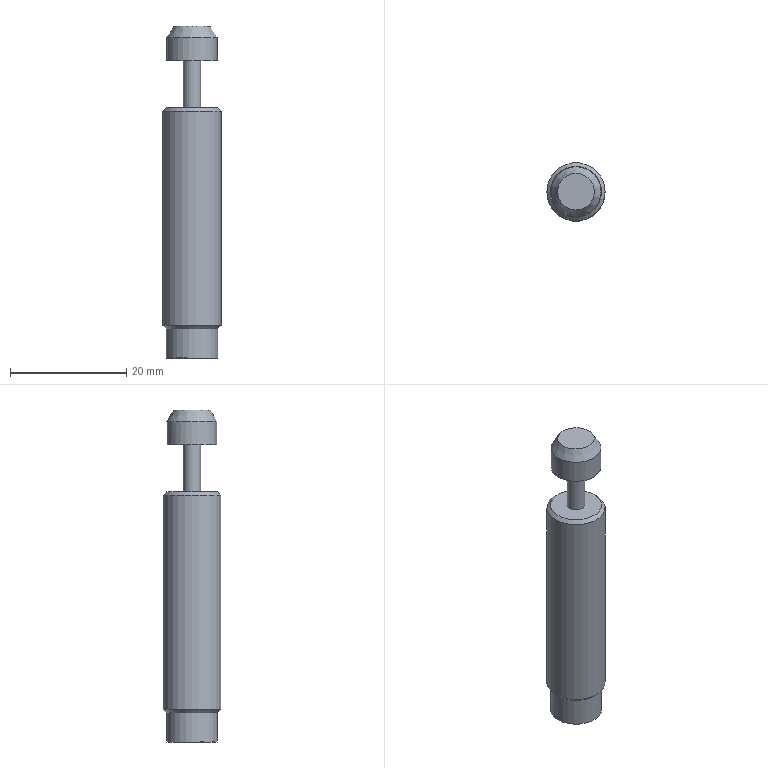Part | NX | 1 solid | 11 faces | box 10 x 10 x 57 mm | volume 3652 mm3 | cylinder 4 | plane 4 | cone 3 | commonest cylinder face diameters 3 x1 8.6 x1 8.773 x1 10 x1
STEP:
#1=CARTESIAN_POINT('',(-5.,0.,-0.6135));
#2=VERTEX_POINT('',#1);
#3=CARTESIAN_POINT('',(0.,0.,-0.6135));
#4=DIRECTION('',(0.,0.,1.));
#5=DIRECTION('',(1.,0.,0.));
#6=AXIS2_PLACEMENT_3D('',#3,#4,#5);
#7=CIRCLE('',#6,5.);
#8=EDGE_CURVE('',#2,#2,#7,.F.);
#9=ORIENTED_EDGE('',*,*,#8,.T.);
#10=EDGE_LOOP('',(#9));
#11=FACE_BOUND('',#10,.T.);
#12=CARTESIAN_POINT('',(-5.,0.,-37.386));
#13=VERTEX_POINT('',#12);
#14=CARTESIAN_POINT('',(0.,0.,-37.386));
#15=DIRECTION('',(0.,0.,1.));
#16=DIRECTION('',(1.,0.,0.));
#17=AXIS2_PLACEMENT_3D('',#14,#15,#16);
#18=CIRCLE('',#17,5.);
#19=EDGE_CURVE('',#13,#13,#18,.T.);
#20=ORIENTED_EDGE('',*,*,#19,.T.);
#21=EDGE_LOOP('',(#20));
#22=FACE_BOUND('',#21,.T.);
#23=CARTESIAN_POINT('',(0.,0.,-500.));
#24=DIRECTION('',(0.,0.,1.));
#25=DIRECTION('',(1.,0.,0.));
#26=AXIS2_PLACEMENT_3D('',#23,#24,#25);
#27=CYLINDRICAL_SURFACE('',#26,5.);
#28=ADVANCED_FACE('',(#11,#22),#27,.T.);
#29=CARTESIAN_POINT('',(-4.387,0.,0.));
#30=VERTEX_POINT('',#29);
#31=CARTESIAN_POINT('',(0.,0.,0.));
#32=DIRECTION('',(0.,0.,-1.));
#33=DIRECTION('',(-1.,0.,0.));
#34=AXIS2_PLACEMENT_3D('',#31,#32,#33);
#35=CIRCLE('',#34,4.387);
#36=EDGE_CURVE('',#30,#30,#35,.T.);
#37=ORIENTED_EDGE('',*,*,#36,.T.);
#38=EDGE_LOOP('',(#37));
#39=FACE_BOUND('',#38,.T.);
#40=ORIENTED_EDGE('',*,*,#8,.F.);
#41=EDGE_LOOP('',(#40));
#42=FACE_BOUND('',#41,.T.);
#43=CARTESIAN_POINT('',(0.,0.,-0.6135));
#44=DIRECTION('',(0.,0.,-1.));
#45=DIRECTION('',(-1.,0.,0.));
#46=AXIS2_PLACEMENT_3D('',#43,#44,#45);
#47=CONICAL_SURFACE('',#46,5.,0.7854);
#48=ADVANCED_FACE('',(#39,#42),#47,.T.);
#49=ORIENTED_EDGE('',*,*,#19,.F.);
#50=EDGE_LOOP('',(#49));
#51=FACE_BOUND('',#50,.T.);
#52=CARTESIAN_POINT('',(-4.387,0.,-38.));
#53=VERTEX_POINT('',#52);
#54=CARTESIAN_POINT('',(0.,0.,-38.));
#55=DIRECTION('',(0.,0.,1.));
#56=DIRECTION('',(1.,0.,0.));
#57=AXIS2_PLACEMENT_3D('',#54,#55,#56);
#58=CIRCLE('',#57,4.387);
#59=EDGE_CURVE('',#53,#53,#58,.T.);
#60=ORIENTED_EDGE('',*,*,#59,.T.);
#61=EDGE_LOOP('',(#60));
#62=FACE_BOUND('',#61,.T.);
#63=CARTESIAN_POINT('',(0.,0.,-37.386));
#64=DIRECTION('',(0.,0.,1.));
#65=DIRECTION('',(1.,0.,0.));
#66=AXIS2_PLACEMENT_3D('',#63,#64,#65);
#67=CONICAL_SURFACE('',#66,5.,0.7854);
#68=ADVANCED_FACE('',(#51,#62),#67,.T.);
#69=CARTESIAN_POINT('',(1.5,0.,0.));
#70=VERTEX_POINT('',#69);
#71=CARTESIAN_POINT('',(0.,0.,0.));
#72=DIRECTION('',(0.,0.,1.));
#73=DIRECTION('',(1.,0.,0.));
#74=AXIS2_PLACEMENT_3D('',#71,#72,#73);
#75=CIRCLE('',#74,1.5);
#76=EDGE_CURVE('',#70,#70,#75,.T.);
#77=ORIENTED_EDGE('',*,*,#76,.F.);
#78=EDGE_LOOP('',(#77));
#79=FACE_BOUND('',#78,.T.);
#80=ORIENTED_EDGE('',*,*,#36,.F.);
#81=EDGE_LOOP('',(#80));
#82=FACE_BOUND('',#81,.T.);
#83=CARTESIAN_POINT('',(0.,1.5,0.));
#84=DIRECTION('',(0.,0.,-1.));
#85=DIRECTION('',(-1.,0.,0.));
#86=AXIS2_PLACEMENT_3D('',#83,#84,#85);
#87=PLANE('',#86);
#88=ADVANCED_FACE('',(#79,#82),#87,.F.);
#89=ORIENTED_EDGE('',*,*,#59,.F.);
#90=EDGE_LOOP('',(#89));
#91=FACE_BOUND('',#90,.T.);
#92=CARTESIAN_POINT('',(4.386,0.,-43.));
#93=VERTEX_POINT('',#92);
#94=CARTESIAN_POINT('',(0.,0.,-43.));
#95=DIRECTION('',(0.,0.,1.));
#96=DIRECTION('',(1.,0.,0.));
#97=AXIS2_PLACEMENT_3D('',#94,#95,#96);
#98=CIRCLE('',#97,4.386);
#99=EDGE_CURVE('',#93,#93,#98,.T.);
#100=ORIENTED_EDGE('',*,*,#99,.T.);
#101=EDGE_LOOP('',(#100));
#102=FACE_BOUND('',#101,.T.);
#103=CARTESIAN_POINT('',(0.,0.,-500.));
#104=DIRECTION('',(0.,0.,1.));
#105=DIRECTION('',(1.,0.,0.));
#106=AXIS2_PLACEMENT_3D('',#103,#104,#105);
#107=CYLINDRICAL_SURFACE('',#106,4.386);
#108=ADVANCED_FACE('',(#91,#102),#107,.T.);
#109=CARTESIAN_POINT('',(1.5,0.,8.));
#110=VERTEX_POINT('',#109);
#111=CARTESIAN_POINT('',(0.,0.,8.));
#112=DIRECTION('',(0.,0.,1.));
#113=DIRECTION('',(1.,0.,0.));
#114=AXIS2_PLACEMENT_3D('',#111,#112,#113);
#115=CIRCLE('',#114,1.5);
#116=EDGE_CURVE('',#110,#110,#115,.F.);
#117=ORIENTED_EDGE('',*,*,#116,.T.);
#118=EDGE_LOOP('',(#117));
#119=FACE_BOUND('',#118,.T.);
#120=ORIENTED_EDGE('',*,*,#76,.T.);
#121=EDGE_LOOP('',(#120));
#122=FACE_BOUND('',#121,.T.);
#123=CARTESIAN_POINT('',(0.,0.,-500.));
#124=DIRECTION('',(0.,0.,1.));
#125=DIRECTION('',(1.,0.,0.));
#126=AXIS2_PLACEMENT_3D('',#123,#124,#125);
#127=CYLINDRICAL_SURFACE('',#126,1.5);
#128=ADVANCED_FACE('',(#119,#122),#127,.T.);
#129=ORIENTED_EDGE('',*,*,#99,.F.);
#130=EDGE_LOOP('',(#129));
#131=FACE_BOUND('',#130,.T.);
#132=CARTESIAN_POINT('',(0.,4.386,-43.));
#133=DIRECTION('',(0.,0.,1.));
#134=DIRECTION('',(1.,0.,0.));
#135=AXIS2_PLACEMENT_3D('',#132,#133,#134);
#136=PLANE('',#135);
#137=ADVANCED_FACE('',(#131),#136,.F.);
#138=CARTESIAN_POINT('',(4.3,0.,8.));
#139=VERTEX_POINT('',#138);
#140=CARTESIAN_POINT('',(0.,0.,8.));
#141=DIRECTION('',(0.,0.,1.));
#142=DIRECTION('',(1.,0.,0.));
#143=AXIS2_PLACEMENT_3D('',#140,#141,#142);
#144=CIRCLE('',#143,4.3);
#145=EDGE_CURVE('',#139,#139,#144,.T.);
#146=ORIENTED_EDGE('',*,*,#145,.F.);
#147=EDGE_LOOP('',(#146));
#148=FACE_BOUND('',#147,.T.);
#149=ORIENTED_EDGE('',*,*,#116,.F.);
#150=EDGE_LOOP('',(#149));
#151=FACE_BOUND('',#150,.T.);
#152=CARTESIAN_POINT('',(0.,4.3,8.));
#153=DIRECTION('',(0.,0.,1.));
#154=DIRECTION('',(1.,0.,0.));
#155=AXIS2_PLACEMENT_3D('',#152,#153,#154);
#156=PLANE('',#155);
#157=ADVANCED_FACE('',(#148,#151),#156,.F.);
#158=CARTESIAN_POINT('',(-4.3,0.,12.));
#159=VERTEX_POINT('',#158);
#160=CARTESIAN_POINT('',(0.,0.,12.));
#161=DIRECTION('',(0.,0.,1.));
#162=DIRECTION('',(1.,0.,0.));
#163=AXIS2_PLACEMENT_3D('',#160,#161,#162);
#164=CIRCLE('',#163,4.3);
#165=EDGE_CURVE('',#159,#159,#164,.F.);
#166=ORIENTED_EDGE('',*,*,#165,.T.);
#167=EDGE_LOOP('',(#166));
#168=FACE_BOUND('',#167,.T.);
#169=ORIENTED_EDGE('',*,*,#145,.T.);
#170=EDGE_LOOP('',(#169));
#171=FACE_BOUND('',#170,.T.);
#172=CARTESIAN_POINT('',(0.,0.,-500.));
#173=DIRECTION('',(0.,0.,1.));
#174=DIRECTION('',(1.,0.,0.));
#175=AXIS2_PLACEMENT_3D('',#172,#173,#174);
#176=CYLINDRICAL_SURFACE('',#175,4.3);
#177=ADVANCED_FACE('',(#168,#171),#176,.T.);
#178=CARTESIAN_POINT('',(0.,3.145,14.));
#179=VERTEX_POINT('',#178);
#180=CARTESIAN_POINT('',(0.,0.,14.));
#181=DIRECTION('',(0.,0.,-1.));
#182=DIRECTION('',(0.,1.,0.));
#183=AXIS2_PLACEMENT_3D('',#180,#181,#182);
#184=CIRCLE('',#183,3.145);
#185=EDGE_CURVE('',#179,#179,#184,.T.);
#186=ORIENTED_EDGE('',*,*,#185,.T.);
#187=EDGE_LOOP('',(#186));
#188=FACE_BOUND('',#187,.T.);
#189=ORIENTED_EDGE('',*,*,#165,.F.);
#190=EDGE_LOOP('',(#189));
#191=FACE_BOUND('',#190,.T.);
#192=CARTESIAN_POINT('',(0.,0.,12.));
#193=DIRECTION('',(0.,0.,-1.));
#194=DIRECTION('',(0.,1.,0.));
#195=AXIS2_PLACEMENT_3D('',#192,#193,#194);
#196=CONICAL_SURFACE('',#195,4.3,0.5236);
#197=ADVANCED_FACE('',(#188,#191),#196,.T.);
#198=ORIENTED_EDGE('',*,*,#185,.F.);
#199=EDGE_LOOP('',(#198));
#200=FACE_BOUND('',#199,.T.);
#201=CARTESIAN_POINT('',(0.,0.,14.));
#202=DIRECTION('',(0.,0.,-1.));
#203=DIRECTION('',(-1.,0.,0.));
#204=AXIS2_PLACEMENT_3D('',#201,#202,#203);
#205=PLANE('',#204);
#206=ADVANCED_FACE('',(#200),#205,.F.);
#207=CLOSED_SHELL('',(#28,#48,#68,#88,#108,#128,#137,#157,#177,#197,#206));
#208=MANIFOLD_SOLID_BREP('',#207);
#209=(LENGTH_UNIT()NAMED_UNIT(*)SI_UNIT(.MILLI.,.METRE.));
#210=UNCERTAINTY_MEASURE_WITH_UNIT(LENGTH_MEASURE(0.00001),#209,'','');
#211=(NAMED_UNIT(*)PLANE_ANGLE_UNIT()SI_UNIT($,.RADIAN.));
#212=(NAMED_UNIT(*)SI_UNIT($,.STERADIAN.)SOLID_ANGLE_UNIT());
#213=(GEOMETRIC_REPRESENTATION_CONTEXT(3)GLOBAL_UNCERTAINTY_ASSIGNED_CONTEXT((#210))GLOBAL_UNIT_ASSIGNED_CONTEXT((#209,#211,#212))REPRESENTATION_CONTEXT('',''));
#214=ADVANCED_BREP_SHAPE_REPRESENTATION('',(#208),#213);